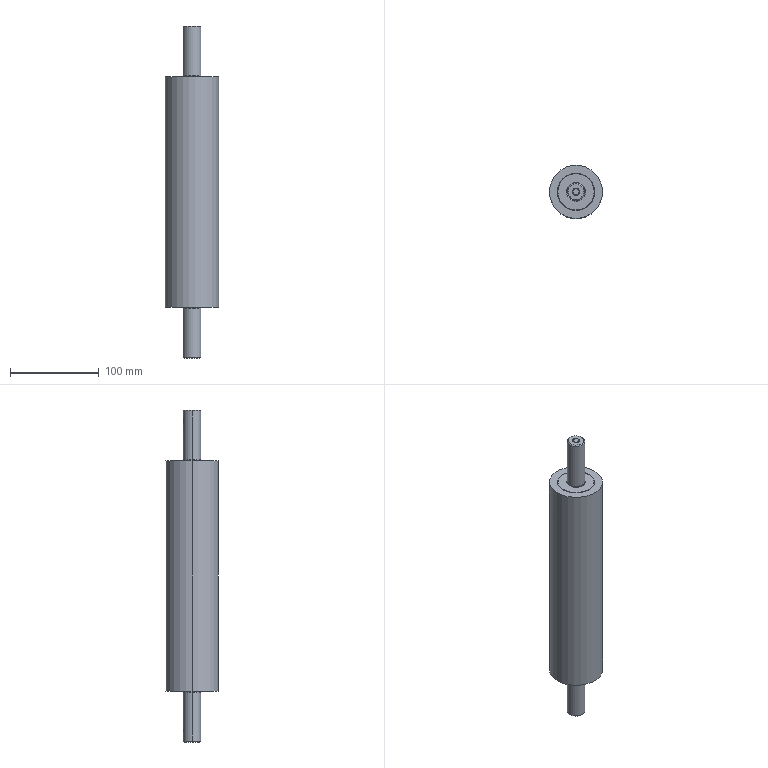Part | SolidWorks | 3 solids | 94 faces | box 60 x 60 x 375 mm | volume 434095 mm3 | cylinder 42 | plane 28 | cone 24 | commonest cylinder face diameters 20 x10 42 x8 6 x6 8 x6 6.8 x4 18.5 x4